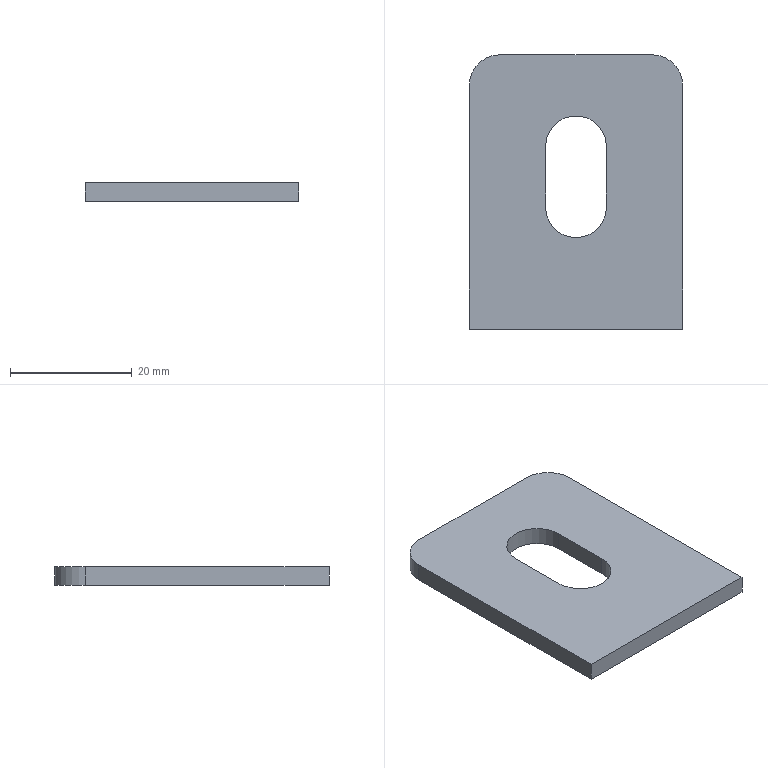Part | SolidWorks | features Extrusion 1 | 1 solid | 12 faces | box 35 x 45 x 3 mm | volume 4157 mm3 | plane 8 | cylinder 4 | commonest cylinder face diameters 10 x4
STEP:
#1=CARTESIAN_POINT('',(0.,40.,3.));
#2=VERTEX_POINT('',#1);
#3=CARTESIAN_POINT('',(0.,0.,3.));
#4=VERTEX_POINT('',#3);
#5=CARTESIAN_POINT('',(0.,0.,3.));
#6=DIRECTION('',(0.,-1.,0.));
#7=VECTOR('',#6,1000.);
#8=LINE('',#5,#7);
#9=EDGE_CURVE('',#2,#4,#8,.T.);
#10=ORIENTED_EDGE('',*,*,#9,.T.);
#11=CARTESIAN_POINT('',(35.,0.,3.));
#12=VERTEX_POINT('',#11);
#13=CARTESIAN_POINT('',(0.,0.,3.));
#14=DIRECTION('',(1.,0.,0.));
#15=VECTOR('',#14,1000.);
#16=LINE('',#13,#15);
#17=EDGE_CURVE('',#4,#12,#16,.T.);
#18=ORIENTED_EDGE('',*,*,#17,.T.);
#19=CARTESIAN_POINT('',(35.,40.,3.));
#20=VERTEX_POINT('',#19);
#21=CARTESIAN_POINT('',(35.,0.,3.));
#22=DIRECTION('',(0.,1.,0.));
#23=VECTOR('',#22,1000.);
#24=LINE('',#21,#23);
#25=EDGE_CURVE('',#12,#20,#24,.T.);
#26=ORIENTED_EDGE('',*,*,#25,.T.);
#27=CARTESIAN_POINT('',(30.,45.,3.));
#28=VERTEX_POINT('',#27);
#29=CARTESIAN_POINT('',(30.,40.,3.));
#30=DIRECTION('',(0.,0.,1.));
#31=DIRECTION('',(-1.,0.,0.));
#32=AXIS2_PLACEMENT_3D('',#29,#30,#31);
#33=CIRCLE('',#32,5.);
#34=EDGE_CURVE('',#20,#28,#33,.T.);
#35=ORIENTED_EDGE('',*,*,#34,.T.);
#36=CARTESIAN_POINT('',(5.,45.,3.));
#37=VERTEX_POINT('',#36);
#38=CARTESIAN_POINT('',(5.,45.,3.));
#39=DIRECTION('',(-1.,0.,0.));
#40=VECTOR('',#39,1000.);
#41=LINE('',#38,#40);
#42=EDGE_CURVE('',#28,#37,#41,.T.);
#43=ORIENTED_EDGE('',*,*,#42,.T.);
#44=CARTESIAN_POINT('',(5.,40.,3.));
#45=DIRECTION('',(0.,0.,1.));
#46=DIRECTION('',(-1.,0.,0.));
#47=AXIS2_PLACEMENT_3D('',#44,#45,#46);
#48=CIRCLE('',#47,5.);
#49=EDGE_CURVE('',#37,#2,#48,.T.);
#50=ORIENTED_EDGE('',*,*,#49,.T.);
#51=EDGE_LOOP('',(#10,#18,#26,#35,#43,#50));
#52=FACE_OUTER_BOUND('',#51,.T.);
#53=CARTESIAN_POINT('',(22.5,30.,3.));
#54=VERTEX_POINT('',#53);
#55=CARTESIAN_POINT('',(12.5,30.,3.));
#56=VERTEX_POINT('',#55);
#57=CARTESIAN_POINT('',(17.5,30.,3.));
#58=DIRECTION('',(0.,0.,1.));
#59=DIRECTION('',(1.,0.,0.));
#60=AXIS2_PLACEMENT_3D('',#57,#58,#59);
#61=CIRCLE('',#60,5.);
#62=EDGE_CURVE('',#54,#56,#61,.T.);
#63=ORIENTED_EDGE('',*,*,#62,.F.);
#64=CARTESIAN_POINT('',(22.5,20.,3.));
#65=VERTEX_POINT('',#64);
#66=CARTESIAN_POINT('',(22.5,30.,3.));
#67=DIRECTION('',(0.,1.,0.));
#68=VECTOR('',#67,1000.);
#69=LINE('',#66,#68);
#70=EDGE_CURVE('',#65,#54,#69,.T.);
#71=ORIENTED_EDGE('',*,*,#70,.F.);
#72=CARTESIAN_POINT('',(12.5,20.,3.));
#73=VERTEX_POINT('',#72);
#74=CARTESIAN_POINT('',(17.5,20.,3.));
#75=DIRECTION('',(0.,0.,1.));
#76=DIRECTION('',(1.,0.,0.));
#77=AXIS2_PLACEMENT_3D('',#74,#75,#76);
#78=CIRCLE('',#77,5.);
#79=EDGE_CURVE('',#73,#65,#78,.T.);
#80=ORIENTED_EDGE('',*,*,#79,.F.);
#81=CARTESIAN_POINT('',(12.5,30.,3.));
#82=DIRECTION('',(0.,-1.,0.));
#83=VECTOR('',#82,1000.);
#84=LINE('',#81,#83);
#85=EDGE_CURVE('',#56,#73,#84,.T.);
#86=ORIENTED_EDGE('',*,*,#85,.F.);
#87=EDGE_LOOP('',(#63,#71,#80,#86));
#88=FACE_BOUND('',#87,.T.);
#89=CARTESIAN_POINT('',(5.,40.,3.));
#90=DIRECTION('',(0.,0.,-1.));
#91=DIRECTION('',(-1.,0.,0.));
#92=AXIS2_PLACEMENT_3D('',#89,#90,#91);
#93=PLANE('',#92);
#94=ADVANCED_FACE('',(#52,#88),#93,.F.);
#95=CARTESIAN_POINT('',(0.,40.,0.));
#96=VERTEX_POINT('',#95);
#97=CARTESIAN_POINT('',(0.,0.,0.));
#98=VERTEX_POINT('',#97);
#99=CARTESIAN_POINT('',(0.,0.,0.));
#100=DIRECTION('',(0.,-1.,0.));
#101=VECTOR('',#100,1000.);
#102=LINE('',#99,#101);
#103=EDGE_CURVE('',#96,#98,#102,.T.);
#104=ORIENTED_EDGE('',*,*,#103,.F.);
#105=CARTESIAN_POINT('',(5.,45.,0.));
#106=VERTEX_POINT('',#105);
#107=CARTESIAN_POINT('',(5.,40.,0.));
#108=DIRECTION('',(0.,0.,1.));
#109=DIRECTION('',(-1.,0.,0.));
#110=AXIS2_PLACEMENT_3D('',#107,#108,#109);
#111=CIRCLE('',#110,5.);
#112=EDGE_CURVE('',#106,#96,#111,.T.);
#113=ORIENTED_EDGE('',*,*,#112,.F.);
#114=CARTESIAN_POINT('',(30.,45.,0.));
#115=VERTEX_POINT('',#114);
#116=CARTESIAN_POINT('',(5.,45.,0.));
#117=DIRECTION('',(-1.,0.,0.));
#118=VECTOR('',#117,1000.);
#119=LINE('',#116,#118);
#120=EDGE_CURVE('',#115,#106,#119,.T.);
#121=ORIENTED_EDGE('',*,*,#120,.F.);
#122=CARTESIAN_POINT('',(35.,40.,0.));
#123=VERTEX_POINT('',#122);
#124=CARTESIAN_POINT('',(30.,40.,0.));
#125=DIRECTION('',(0.,0.,1.));
#126=DIRECTION('',(-1.,0.,0.));
#127=AXIS2_PLACEMENT_3D('',#124,#125,#126);
#128=CIRCLE('',#127,5.);
#129=EDGE_CURVE('',#123,#115,#128,.T.);
#130=ORIENTED_EDGE('',*,*,#129,.F.);
#131=CARTESIAN_POINT('',(35.,0.,0.));
#132=VERTEX_POINT('',#131);
#133=CARTESIAN_POINT('',(35.,0.,0.));
#134=DIRECTION('',(0.,1.,0.));
#135=VECTOR('',#134,1000.);
#136=LINE('',#133,#135);
#137=EDGE_CURVE('',#132,#123,#136,.T.);
#138=ORIENTED_EDGE('',*,*,#137,.F.);
#139=CARTESIAN_POINT('',(0.,0.,0.));
#140=DIRECTION('',(1.,0.,0.));
#141=VECTOR('',#140,1000.);
#142=LINE('',#139,#141);
#143=EDGE_CURVE('',#98,#132,#142,.T.);
#144=ORIENTED_EDGE('',*,*,#143,.F.);
#145=EDGE_LOOP('',(#104,#113,#121,#130,#138,#144));
#146=FACE_OUTER_BOUND('',#145,.T.);
#147=CARTESIAN_POINT('',(22.5,20.,0.));
#148=VERTEX_POINT('',#147);
#149=CARTESIAN_POINT('',(22.5,30.,0.));
#150=VERTEX_POINT('',#149);
#151=CARTESIAN_POINT('',(22.5,30.,0.));
#152=DIRECTION('',(0.,1.,0.));
#153=VECTOR('',#152,1000.);
#154=LINE('',#151,#153);
#155=EDGE_CURVE('',#148,#150,#154,.T.);
#156=ORIENTED_EDGE('',*,*,#155,.T.);
#157=CARTESIAN_POINT('',(12.5,30.,0.));
#158=VERTEX_POINT('',#157);
#159=CARTESIAN_POINT('',(17.5,30.,0.));
#160=DIRECTION('',(0.,0.,1.));
#161=DIRECTION('',(1.,0.,0.));
#162=AXIS2_PLACEMENT_3D('',#159,#160,#161);
#163=CIRCLE('',#162,5.);
#164=EDGE_CURVE('',#150,#158,#163,.T.);
#165=ORIENTED_EDGE('',*,*,#164,.T.);
#166=CARTESIAN_POINT('',(12.5,20.,0.));
#167=VERTEX_POINT('',#166);
#168=CARTESIAN_POINT('',(12.5,30.,0.));
#169=DIRECTION('',(0.,-1.,0.));
#170=VECTOR('',#169,1000.);
#171=LINE('',#168,#170);
#172=EDGE_CURVE('',#158,#167,#171,.T.);
#173=ORIENTED_EDGE('',*,*,#172,.T.);
#174=CARTESIAN_POINT('',(17.5,20.,0.));
#175=DIRECTION('',(0.,0.,1.));
#176=DIRECTION('',(1.,0.,0.));
#177=AXIS2_PLACEMENT_3D('',#174,#175,#176);
#178=CIRCLE('',#177,5.);
#179=EDGE_CURVE('',#167,#148,#178,.T.);
#180=ORIENTED_EDGE('',*,*,#179,.T.);
#181=EDGE_LOOP('',(#156,#165,#173,#180));
#182=FACE_BOUND('',#181,.T.);
#183=CARTESIAN_POINT('',(5.,40.,0.));
#184=DIRECTION('',(0.,0.,-1.));
#185=DIRECTION('',(-1.,0.,0.));
#186=AXIS2_PLACEMENT_3D('',#183,#184,#185);
#187=PLANE('',#186);
#188=ADVANCED_FACE('',(#146,#182),#187,.T.);
#189=ORIENTED_EDGE('',*,*,#103,.T.);
#190=CARTESIAN_POINT('',(0.,0.,3.));
#191=DIRECTION('',(0.,0.,-1.));
#192=VECTOR('',#191,1000.);
#193=LINE('',#190,#192);
#194=EDGE_CURVE('',#4,#98,#193,.T.);
#195=ORIENTED_EDGE('',*,*,#194,.F.);
#196=ORIENTED_EDGE('',*,*,#9,.F.);
#197=CARTESIAN_POINT('',(0.,40.,3.));
#198=DIRECTION('',(0.,0.,-1.));
#199=VECTOR('',#198,1000.);
#200=LINE('',#197,#199);
#201=EDGE_CURVE('',#2,#96,#200,.T.);
#202=ORIENTED_EDGE('',*,*,#201,.T.);
#203=EDGE_LOOP('',(#189,#195,#196,#202));
#204=FACE_OUTER_BOUND('',#203,.T.);
#205=CARTESIAN_POINT('',(0.,0.,3.));
#206=DIRECTION('',(1.,0.,0.));
#207=DIRECTION('',(0.,0.,-1.));
#208=AXIS2_PLACEMENT_3D('',#205,#206,#207);
#209=PLANE('',#208);
#210=ADVANCED_FACE('',(#204),#209,.F.);
#211=ORIENTED_EDGE('',*,*,#143,.T.);
#212=CARTESIAN_POINT('',(35.,0.,3.));
#213=DIRECTION('',(0.,0.,-1.));
#214=VECTOR('',#213,1000.);
#215=LINE('',#212,#214);
#216=EDGE_CURVE('',#12,#132,#215,.T.);
#217=ORIENTED_EDGE('',*,*,#216,.F.);
#218=ORIENTED_EDGE('',*,*,#17,.F.);
#219=ORIENTED_EDGE('',*,*,#194,.T.);
#220=EDGE_LOOP('',(#211,#217,#218,#219));
#221=FACE_OUTER_BOUND('',#220,.T.);
#222=CARTESIAN_POINT('',(0.,0.,3.));
#223=DIRECTION('',(0.,1.,0.));
#224=DIRECTION('',(0.,0.,1.));
#225=AXIS2_PLACEMENT_3D('',#222,#223,#224);
#226=PLANE('',#225);
#227=ADVANCED_FACE('',(#221),#226,.F.);
#228=ORIENTED_EDGE('',*,*,#137,.T.);
#229=CARTESIAN_POINT('',(35.,40.,3.));
#230=DIRECTION('',(0.,0.,-1.));
#231=VECTOR('',#230,1000.);
#232=LINE('',#229,#231);
#233=EDGE_CURVE('',#20,#123,#232,.T.);
#234=ORIENTED_EDGE('',*,*,#233,.F.);
#235=ORIENTED_EDGE('',*,*,#25,.F.);
#236=ORIENTED_EDGE('',*,*,#216,.T.);
#237=EDGE_LOOP('',(#228,#234,#235,#236));
#238=FACE_OUTER_BOUND('',#237,.T.);
#239=CARTESIAN_POINT('',(35.,0.,3.));
#240=DIRECTION('',(-1.,0.,0.));
#241=DIRECTION('',(0.,0.,1.));
#242=AXIS2_PLACEMENT_3D('',#239,#240,#241);
#243=PLANE('',#242);
#244=ADVANCED_FACE('',(#238),#243,.F.);
#245=ORIENTED_EDGE('',*,*,#129,.T.);
#246=CARTESIAN_POINT('',(30.,45.,3.));
#247=DIRECTION('',(0.,0.,-1.));
#248=VECTOR('',#247,1000.);
#249=LINE('',#246,#248);
#250=EDGE_CURVE('',#28,#115,#249,.T.);
#251=ORIENTED_EDGE('',*,*,#250,.F.);
#252=ORIENTED_EDGE('',*,*,#34,.F.);
#253=ORIENTED_EDGE('',*,*,#233,.T.);
#254=EDGE_LOOP('',(#245,#251,#252,#253));
#255=FACE_OUTER_BOUND('',#254,.T.);
#256=CARTESIAN_POINT('',(30.,40.,3.));
#257=DIRECTION('',(0.,0.,-1.));
#258=DIRECTION('',(-1.,0.,0.));
#259=AXIS2_PLACEMENT_3D('',#256,#257,#258);
#260=CYLINDRICAL_SURFACE('',#259,5.);
#261=ADVANCED_FACE('',(#255),#260,.T.);
#262=ORIENTED_EDGE('',*,*,#120,.T.);
#263=CARTESIAN_POINT('',(5.,45.,3.));
#264=DIRECTION('',(0.,0.,-1.));
#265=VECTOR('',#264,1000.);
#266=LINE('',#263,#265);
#267=EDGE_CURVE('',#37,#106,#266,.T.);
#268=ORIENTED_EDGE('',*,*,#267,.F.);
#269=ORIENTED_EDGE('',*,*,#42,.F.);
#270=ORIENTED_EDGE('',*,*,#250,.T.);
#271=EDGE_LOOP('',(#262,#268,#269,#270));
#272=FACE_OUTER_BOUND('',#271,.T.);
#273=CARTESIAN_POINT('',(5.,45.,3.));
#274=DIRECTION('',(0.,-1.,0.));
#275=DIRECTION('',(0.,0.,-1.));
#276=AXIS2_PLACEMENT_3D('',#273,#274,#275);
#277=PLANE('',#276);
#278=ADVANCED_FACE('',(#272),#277,.F.);
#279=ORIENTED_EDGE('',*,*,#112,.T.);
#280=ORIENTED_EDGE('',*,*,#201,.F.);
#281=ORIENTED_EDGE('',*,*,#49,.F.);
#282=ORIENTED_EDGE('',*,*,#267,.T.);
#283=EDGE_LOOP('',(#279,#280,#281,#282));
#284=FACE_OUTER_BOUND('',#283,.T.);
#285=CARTESIAN_POINT('',(5.,40.,3.));
#286=DIRECTION('',(0.,0.,-1.));
#287=DIRECTION('',(-1.,0.,0.));
#288=AXIS2_PLACEMENT_3D('',#285,#286,#287);
#289=CYLINDRICAL_SURFACE('',#288,5.);
#290=ADVANCED_FACE('',(#284),#289,.T.);
#291=ORIENTED_EDGE('',*,*,#164,.F.);
#292=CARTESIAN_POINT('',(22.5,30.,3.));
#293=DIRECTION('',(0.,0.,-1.));
#294=VECTOR('',#293,1000.);
#295=LINE('',#292,#294);
#296=EDGE_CURVE('',#54,#150,#295,.T.);
#297=ORIENTED_EDGE('',*,*,#296,.F.);
#298=ORIENTED_EDGE('',*,*,#62,.T.);
#299=CARTESIAN_POINT('',(12.5,30.,3.));
#300=DIRECTION('',(0.,0.,-1.));
#301=VECTOR('',#300,1000.);
#302=LINE('',#299,#301);
#303=EDGE_CURVE('',#56,#158,#302,.T.);
#304=ORIENTED_EDGE('',*,*,#303,.T.);
#305=EDGE_LOOP('',(#291,#297,#298,#304));
#306=FACE_OUTER_BOUND('',#305,.T.);
#307=CARTESIAN_POINT('',(17.5,30.,3.));
#308=DIRECTION('',(0.,0.,-1.));
#309=DIRECTION('',(-1.,0.,0.));
#310=AXIS2_PLACEMENT_3D('',#307,#308,#309);
#311=CYLINDRICAL_SURFACE('',#310,5.);
#312=ADVANCED_FACE('',(#306),#311,.F.);
#313=ORIENTED_EDGE('',*,*,#172,.F.);
#314=ORIENTED_EDGE('',*,*,#303,.F.);
#315=ORIENTED_EDGE('',*,*,#85,.T.);
#316=CARTESIAN_POINT('',(12.5,20.,3.));
#317=DIRECTION('',(0.,0.,-1.));
#318=VECTOR('',#317,1000.);
#319=LINE('',#316,#318);
#320=EDGE_CURVE('',#73,#167,#319,.T.);
#321=ORIENTED_EDGE('',*,*,#320,.T.);
#322=EDGE_LOOP('',(#313,#314,#315,#321));
#323=FACE_OUTER_BOUND('',#322,.T.);
#324=CARTESIAN_POINT('',(12.5,30.,3.));
#325=DIRECTION('',(1.,0.,0.));
#326=DIRECTION('',(0.,0.,-1.));
#327=AXIS2_PLACEMENT_3D('',#324,#325,#326);
#328=PLANE('',#327);
#329=ADVANCED_FACE('',(#323),#328,.T.);
#330=ORIENTED_EDGE('',*,*,#179,.F.);
#331=ORIENTED_EDGE('',*,*,#320,.F.);
#332=ORIENTED_EDGE('',*,*,#79,.T.);
#333=CARTESIAN_POINT('',(22.5,20.,3.));
#334=DIRECTION('',(0.,0.,-1.));
#335=VECTOR('',#334,1000.);
#336=LINE('',#333,#335);
#337=EDGE_CURVE('',#65,#148,#336,.T.);
#338=ORIENTED_EDGE('',*,*,#337,.T.);
#339=EDGE_LOOP('',(#330,#331,#332,#338));
#340=FACE_OUTER_BOUND('',#339,.T.);
#341=CARTESIAN_POINT('',(17.5,20.,3.));
#342=DIRECTION('',(0.,0.,-1.));
#343=DIRECTION('',(-1.,0.,0.));
#344=AXIS2_PLACEMENT_3D('',#341,#342,#343);
#345=CYLINDRICAL_SURFACE('',#344,5.);
#346=ADVANCED_FACE('',(#340),#345,.F.);
#347=ORIENTED_EDGE('',*,*,#155,.F.);
#348=ORIENTED_EDGE('',*,*,#337,.F.);
#349=ORIENTED_EDGE('',*,*,#70,.T.);
#350=ORIENTED_EDGE('',*,*,#296,.T.);
#351=EDGE_LOOP('',(#347,#348,#349,#350));
#352=FACE_OUTER_BOUND('',#351,.T.);
#353=CARTESIAN_POINT('',(22.5,30.,3.));
#354=DIRECTION('',(-1.,0.,0.));
#355=DIRECTION('',(0.,0.,1.));
#356=AXIS2_PLACEMENT_3D('',#353,#354,#355);
#357=PLANE('',#356);
#358=ADVANCED_FACE('',(#352),#357,.T.);
#359=CLOSED_SHELL('',(#94,#188,#210,#227,#244,#261,#278,#290,#312,#329,#346,#358));
#360=MANIFOLD_SOLID_BREP('',#359);
#361=CARTESIAN_POINT('',(0.,0.,0.));
#362=DIRECTION('',(0.,0.,1.));
#363=DIRECTION('',(1.,0.,0.));
#364=AXIS2_PLACEMENT_3D('',#361,#362,#363);
#365=(LENGTH_UNIT()NAMED_UNIT(*)SI_UNIT(.MILLI.,.METRE.));
#366=UNCERTAINTY_MEASURE_WITH_UNIT(LENGTH_MEASURE(0.00001),#365,'','');
#367=(NAMED_UNIT(*)PLANE_ANGLE_UNIT()SI_UNIT($,.RADIAN.));
#368=(NAMED_UNIT(*)SI_UNIT($,.STERADIAN.)SOLID_ANGLE_UNIT());
#369=(GEOMETRIC_REPRESENTATION_CONTEXT(3)GLOBAL_UNCERTAINTY_ASSIGNED_CONTEXT((#366))GLOBAL_UNIT_ASSIGNED_CONTEXT((#365,#367,#368))REPRESENTATION_CONTEXT('',''));
#370=ADVANCED_BREP_SHAPE_REPRESENTATION('',(#360,#364),#369);